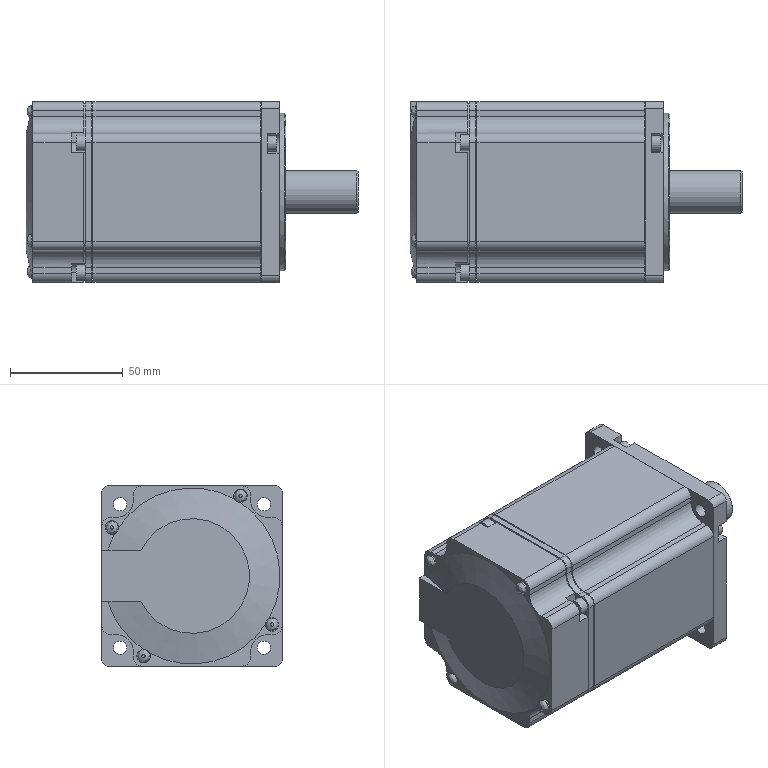Part | NX | 1 solid | 239 faces | box 147.2 x 80 x 80 mm | volume 647434 mm3 | plane 131 | cylinder 101 | spline 4 | cone 3 | commonest cylinder face diameters 8 x44 15 x24 6 x12 7 x8 8.5 x8 19 x1